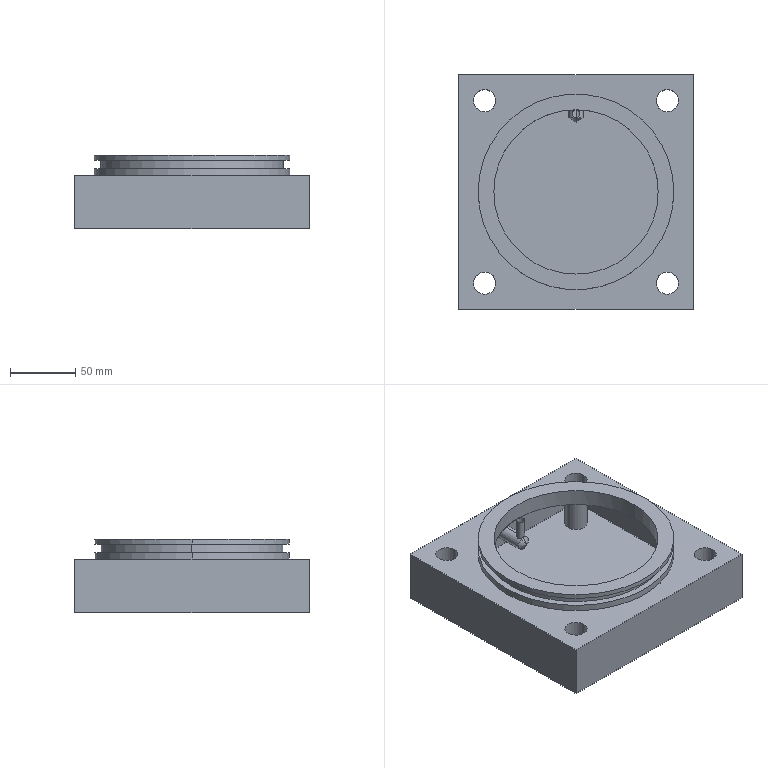Part | SolidWorks | features ICE 4, Extrusion 1, HoleWzd 1, RevCut 1 | 1 solid | 35 faces | box 180 x 180 x 56 mm | volume 1375420 mm3 | cylinder 20 | plane 11 | cone 4 | commonest cylinder face diameters 17 x8 150 x4 6 x2 11.125 x2 126 x2 140 x2
STEP:
#1=CARTESIAN_POINT('',(61.5,-70.,41.));
#2=VERTEX_POINT('',#1);
#3=CARTESIAN_POINT('',(78.5,-70.,41.));
#4=VERTEX_POINT('',#3);
#5=CARTESIAN_POINT('',(70.,-70.,41.));
#6=DIRECTION('',(0.,0.,1.));
#7=DIRECTION('',(-1.,0.,0.));
#8=AXIS2_PLACEMENT_3D('',#5,#6,#7);
#9=CIRCLE('',#8,8.5);
#10=EDGE_CURVE('',#2,#4,#9,.T.);
#11=ORIENTED_EDGE('',*,*,#10,.T.);
#12=CARTESIAN_POINT('',(78.5,-70.,0.));
#13=VERTEX_POINT('',#12);
#14=CARTESIAN_POINT('',(78.5,-70.,56.001));
#15=DIRECTION('',(0.,0.,-1.));
#16=VECTOR('',#15,1000.);
#17=LINE('',#14,#16);
#18=EDGE_CURVE('',#4,#13,#17,.T.);
#19=ORIENTED_EDGE('',*,*,#18,.T.);
#20=CARTESIAN_POINT('',(61.5,-70.,0.));
#21=VERTEX_POINT('',#20);
#22=CARTESIAN_POINT('',(70.,-70.,0.));
#23=DIRECTION('',(0.,0.,-1.));
#24=DIRECTION('',(-1.,0.,0.));
#25=AXIS2_PLACEMENT_3D('',#22,#23,#24);
#26=CIRCLE('',#25,8.5);
#27=EDGE_CURVE('',#13,#21,#26,.T.);
#28=ORIENTED_EDGE('',*,*,#27,.T.);
#29=CARTESIAN_POINT('',(61.5,-70.,56.001));
#30=DIRECTION('',(0.,0.,-1.));
#31=VECTOR('',#30,1000.);
#32=LINE('',#29,#31);
#33=EDGE_CURVE('',#2,#21,#32,.T.);
#34=ORIENTED_EDGE('',*,*,#33,.F.);
#35=EDGE_LOOP('',(#11,#19,#28,#34));
#36=FACE_OUTER_BOUND('',#35,.T.);
#37=CARTESIAN_POINT('',(70.,-70.,56.001));
#38=DIRECTION('',(0.,0.,-1.));
#39=DIRECTION('',(-1.,0.,0.));
#40=AXIS2_PLACEMENT_3D('',#37,#38,#39);
#41=CYLINDRICAL_SURFACE('',#40,8.5);
#42=ADVANCED_FACE('',(#36),#41,.F.);
#43=CARTESIAN_POINT('',(-78.5,-70.,41.));
#44=VERTEX_POINT('',#43);
#45=CARTESIAN_POINT('',(-61.5,-70.,41.));
#46=VERTEX_POINT('',#45);
#47=CARTESIAN_POINT('',(-70.,-70.,41.));
#48=DIRECTION('',(0.,0.,1.));
#49=DIRECTION('',(-1.,0.,0.));
#50=AXIS2_PLACEMENT_3D('',#47,#48,#49);
#51=CIRCLE('',#50,8.5);
#52=EDGE_CURVE('',#44,#46,#51,.T.);
#53=ORIENTED_EDGE('',*,*,#52,.T.);
#54=CARTESIAN_POINT('',(-61.5,-70.,0.));
#55=VERTEX_POINT('',#54);
#56=CARTESIAN_POINT('',(-61.5,-70.,56.001));
#57=DIRECTION('',(0.,0.,-1.));
#58=VECTOR('',#57,1000.);
#59=LINE('',#56,#58);
#60=EDGE_CURVE('',#46,#55,#59,.T.);
#61=ORIENTED_EDGE('',*,*,#60,.T.);
#62=CARTESIAN_POINT('',(-78.5,-70.,0.));
#63=VERTEX_POINT('',#62);
#64=CARTESIAN_POINT('',(-70.,-70.,0.));
#65=DIRECTION('',(0.,0.,-1.));
#66=DIRECTION('',(-1.,0.,0.));
#67=AXIS2_PLACEMENT_3D('',#64,#65,#66);
#68=CIRCLE('',#67,8.5);
#69=EDGE_CURVE('',#55,#63,#68,.T.);
#70=ORIENTED_EDGE('',*,*,#69,.T.);
#71=CARTESIAN_POINT('',(-78.5,-70.,56.001));
#72=DIRECTION('',(0.,0.,-1.));
#73=VECTOR('',#72,1000.);
#74=LINE('',#71,#73);
#75=EDGE_CURVE('',#44,#63,#74,.T.);
#76=ORIENTED_EDGE('',*,*,#75,.F.);
#77=EDGE_LOOP('',(#53,#61,#70,#76));
#78=FACE_OUTER_BOUND('',#77,.T.);
#79=CARTESIAN_POINT('',(-70.,-70.,56.001));
#80=DIRECTION('',(0.,0.,-1.));
#81=DIRECTION('',(-1.,0.,0.));
#82=AXIS2_PLACEMENT_3D('',#79,#80,#81);
#83=CYLINDRICAL_SURFACE('',#82,8.5);
#84=ADVANCED_FACE('',(#78),#83,.F.);
#85=CARTESIAN_POINT('',(-78.5,70.,41.));
#86=VERTEX_POINT('',#85);
#87=CARTESIAN_POINT('',(-61.5,70.,41.));
#88=VERTEX_POINT('',#87);
#89=CARTESIAN_POINT('',(-70.,70.,41.));
#90=DIRECTION('',(0.,0.,1.));
#91=DIRECTION('',(-1.,0.,0.));
#92=AXIS2_PLACEMENT_3D('',#89,#90,#91);
#93=CIRCLE('',#92,8.5);
#94=EDGE_CURVE('',#86,#88,#93,.T.);
#95=ORIENTED_EDGE('',*,*,#94,.T.);
#96=CARTESIAN_POINT('',(-61.5,70.,0.));
#97=VERTEX_POINT('',#96);
#98=CARTESIAN_POINT('',(-61.5,70.,56.001));
#99=DIRECTION('',(0.,0.,-1.));
#100=VECTOR('',#99,1000.);
#101=LINE('',#98,#100);
#102=EDGE_CURVE('',#88,#97,#101,.T.);
#103=ORIENTED_EDGE('',*,*,#102,.T.);
#104=CARTESIAN_POINT('',(-78.5,70.,0.));
#105=VERTEX_POINT('',#104);
#106=CARTESIAN_POINT('',(-70.,70.,0.));
#107=DIRECTION('',(0.,0.,-1.));
#108=DIRECTION('',(-1.,0.,0.));
#109=AXIS2_PLACEMENT_3D('',#106,#107,#108);
#110=CIRCLE('',#109,8.5);
#111=EDGE_CURVE('',#97,#105,#110,.T.);
#112=ORIENTED_EDGE('',*,*,#111,.T.);
#113=CARTESIAN_POINT('',(-78.5,70.,56.001));
#114=DIRECTION('',(0.,0.,-1.));
#115=VECTOR('',#114,1000.);
#116=LINE('',#113,#115);
#117=EDGE_CURVE('',#86,#105,#116,.T.);
#118=ORIENTED_EDGE('',*,*,#117,.F.);
#119=EDGE_LOOP('',(#95,#103,#112,#118));
#120=FACE_OUTER_BOUND('',#119,.T.);
#121=CARTESIAN_POINT('',(-70.,70.,56.001));
#122=DIRECTION('',(0.,0.,-1.));
#123=DIRECTION('',(-1.,0.,0.));
#124=AXIS2_PLACEMENT_3D('',#121,#122,#123);
#125=CYLINDRICAL_SURFACE('',#124,8.5);
#126=ADVANCED_FACE('',(#120),#125,.F.);
#127=CARTESIAN_POINT('',(61.5,70.,41.));
#128=VERTEX_POINT('',#127);
#129=CARTESIAN_POINT('',(78.5,70.,41.));
#130=VERTEX_POINT('',#129);
#131=CARTESIAN_POINT('',(70.,70.,41.));
#132=DIRECTION('',(0.,0.,1.));
#133=DIRECTION('',(-1.,0.,0.));
#134=AXIS2_PLACEMENT_3D('',#131,#132,#133);
#135=CIRCLE('',#134,8.5);
#136=EDGE_CURVE('',#128,#130,#135,.T.);
#137=ORIENTED_EDGE('',*,*,#136,.T.);
#138=CARTESIAN_POINT('',(78.5,70.,0.));
#139=VERTEX_POINT('',#138);
#140=CARTESIAN_POINT('',(78.5,70.,56.001));
#141=DIRECTION('',(0.,0.,-1.));
#142=VECTOR('',#141,1000.);
#143=LINE('',#140,#142);
#144=EDGE_CURVE('',#130,#139,#143,.T.);
#145=ORIENTED_EDGE('',*,*,#144,.T.);
#146=CARTESIAN_POINT('',(61.5,70.,0.));
#147=VERTEX_POINT('',#146);
#148=CARTESIAN_POINT('',(70.,70.,0.));
#149=DIRECTION('',(0.,0.,-1.));
#150=DIRECTION('',(-1.,0.,0.));
#151=AXIS2_PLACEMENT_3D('',#148,#149,#150);
#152=CIRCLE('',#151,8.5);
#153=EDGE_CURVE('',#139,#147,#152,.T.);
#154=ORIENTED_EDGE('',*,*,#153,.T.);
#155=CARTESIAN_POINT('',(61.5,70.,56.001));
#156=DIRECTION('',(0.,0.,-1.));
#157=VECTOR('',#156,1000.);
#158=LINE('',#155,#157);
#159=EDGE_CURVE('',#128,#147,#158,.T.);
#160=ORIENTED_EDGE('',*,*,#159,.F.);
#161=EDGE_LOOP('',(#137,#145,#154,#160));
#162=FACE_OUTER_BOUND('',#161,.T.);
#163=CARTESIAN_POINT('',(70.,70.,56.001));
#164=DIRECTION('',(0.,0.,-1.));
#165=DIRECTION('',(-1.,0.,0.));
#166=AXIS2_PLACEMENT_3D('',#163,#164,#165);
#167=CYLINDRICAL_SURFACE('',#166,8.5);
#168=ADVANCED_FACE('',(#162),#167,.F.);
#169=CARTESIAN_POINT('',(0.,57.,28.563));
#170=VERTEX_POINT('',#169);
#171=CARTESIAN_POINT('',(-3.,60.,27.684));
#172=VERTEX_POINT('',#171);
#173=CARTESIAN_POINT('',(0.,57.,28.563));
#174=CARTESIAN_POINT('',(-0.2027,57.,28.563));
#175=CARTESIAN_POINT('',(-0.4013,57.02,28.552));
#176=CARTESIAN_POINT('',(-0.7909,57.099,28.51));
#177=CARTESIAN_POINT('',(-0.9837,57.159,28.478));
#178=CARTESIAN_POINT('',(-1.527,57.388,28.362));
#179=CARTESIAN_POINT('',(-1.855,57.611,28.253));
#180=CARTESIAN_POINT('',(-2.261,58.019,28.084));
#181=CARTESIAN_POINT('',(-2.385,58.169,28.027));
#182=CARTESIAN_POINT('',(-2.6,58.491,27.919));
#183=CARTESIAN_POINT('',(-2.692,58.661,27.869));
#184=CARTESIAN_POINT('',(-2.842,59.02,27.782));
#185=CARTESIAN_POINT('',(-2.902,59.213,27.746));
#186=CARTESIAN_POINT('',(-2.98,59.602,27.697));
#187=CARTESIAN_POINT('',(-3.,59.799,27.684));
#188=CARTESIAN_POINT('',(-3.,60.,27.684));
#189=B_SPLINE_CURVE_WITH_KNOTS('',3,(#173,#174,#175,#176,#177,#178,#179,#180,#181,#182,#183,#184,#185,#186,#187,#188),.UNSPECIFIED.,.F.,.F.,(4,2,2,2,2,2,2,4),(0.,0.0005988,0.001198,0.002395,0.002994,0.003593,0.004192,0.00479),.UNSPECIFIED.);
#190=EDGE_CURVE('',#170,#172,#189,.T.);
#191=ORIENTED_EDGE('',*,*,#190,.T.);
#192=CARTESIAN_POINT('',(-3.,60.,43.));
#193=VERTEX_POINT('',#192);
#194=CARTESIAN_POINT('',(-3.,60.,-0.001));
#195=DIRECTION('',(0.,0.,1.));
#196=VECTOR('',#195,1000.);
#197=LINE('',#194,#196);
#198=EDGE_CURVE('',#172,#193,#197,.T.);
#199=ORIENTED_EDGE('',*,*,#198,.T.);
#200=CARTESIAN_POINT('',(3.,60.,43.));
#201=VERTEX_POINT('',#200);
#202=CARTESIAN_POINT('',(0.,60.,43.));
#203=DIRECTION('',(0.,0.,1.));
#204=DIRECTION('',(1.,0.,0.));
#205=AXIS2_PLACEMENT_3D('',#202,#203,#204);
#206=CIRCLE('',#205,3.);
#207=EDGE_CURVE('',#193,#201,#206,.T.);
#208=ORIENTED_EDGE('',*,*,#207,.T.);
#209=CARTESIAN_POINT('',(3.,60.,27.684));
#210=VERTEX_POINT('',#209);
#211=CARTESIAN_POINT('',(3.,60.,-0.001));
#212=DIRECTION('',(0.,0.,1.));
#213=VECTOR('',#212,1000.);
#214=LINE('',#211,#213);
#215=EDGE_CURVE('',#210,#201,#214,.T.);
#216=ORIENTED_EDGE('',*,*,#215,.F.);
#217=CARTESIAN_POINT('',(3.,60.,27.684));
#218=CARTESIAN_POINT('',(3.,59.801,27.684));
#219=CARTESIAN_POINT('',(2.98,59.598,27.697));
#220=CARTESIAN_POINT('',(2.901,59.209,27.747));
#221=CARTESIAN_POINT('',(2.843,59.021,27.782));
#222=CARTESIAN_POINT('',(2.69,58.657,27.87));
#223=CARTESIAN_POINT('',(2.597,58.486,27.92));
#224=CARTESIAN_POINT('',(2.382,58.167,28.028));
#225=CARTESIAN_POINT('',(2.258,58.016,28.086));
#226=CARTESIAN_POINT('',(1.987,57.744,28.198));
#227=CARTESIAN_POINT('',(1.839,57.622,28.252));
#228=CARTESIAN_POINT('',(1.518,57.405,28.354));
#229=CARTESIAN_POINT('',(1.344,57.311,28.401));
#230=CARTESIAN_POINT('',(0.9842,57.159,28.478));
#231=CARTESIAN_POINT('',(0.7966,57.101,28.509));
#232=CARTESIAN_POINT('',(0.4039,57.021,28.551));
#233=CARTESIAN_POINT('',(0.2019,57.,28.563));
#234=CARTESIAN_POINT('',(0.,57.,28.563));
#235=B_SPLINE_CURVE_WITH_KNOTS('',3,(#217,#218,#219,#220,#221,#222,#223,#224,#225,#226,#227,#228,#229,#230,#231,#232,#233,#234),.UNSPECIFIED.,.F.,.F.,(4,2,2,2,2,2,2,2,4),(0.01435,0.01495,0.01555,0.01614,0.01674,0.01734,0.01793,0.01853,0.01913),.UNSPECIFIED.);
#236=EDGE_CURVE('',#210,#170,#235,.T.);
#237=ORIENTED_EDGE('',*,*,#236,.T.);
#238=EDGE_LOOP('',(#191,#199,#208,#216,#237));
#239=FACE_OUTER_BOUND('',#238,.T.);
#240=CARTESIAN_POINT('',(0.,60.,-0.001));
#241=DIRECTION('',(0.,0.,1.));
#242=DIRECTION('',(1.,0.,0.));
#243=AXIS2_PLACEMENT_3D('',#240,#241,#242);
#244=CYLINDRICAL_SURFACE('',#243,3.);
#245=ADVANCED_FACE('',(#239),#244,.F.);
#246=CARTESIAN_POINT('',(0.,79.98,17.056));
#247=VERTEX_POINT('',#246);
#248=CARTESIAN_POINT('',(0.,79.98,28.944));
#249=VERTEX_POINT('',#248);
#250=CARTESIAN_POINT('',(0.,79.98,23.));
#251=DIRECTION('',(0.,1.,0.));
#252=DIRECTION('',(0.,0.,1.));
#253=AXIS2_PLACEMENT_3D('',#250,#251,#252);
#254=CIRCLE('',#253,5.944);
#255=EDGE_CURVE('',#247,#249,#254,.T.);
#256=ORIENTED_EDGE('',*,*,#255,.F.);
#257=CARTESIAN_POINT('',(0.,90.,16.756));
#258=VERTEX_POINT('',#257);
#259=CARTESIAN_POINT('',(0.,90.,16.756));
#260=DIRECTION('',(0.,0.9996,-0.02993));
#261=VECTOR('',#260,1000.);
#262=LINE('',#259,#261);
#263=EDGE_CURVE('',#247,#258,#262,.T.);
#264=ORIENTED_EDGE('',*,*,#263,.T.);
#265=CARTESIAN_POINT('',(0.,90.,29.244));
#266=VERTEX_POINT('',#265);
#267=CARTESIAN_POINT('',(0.,90.,23.));
#268=DIRECTION('',(0.,1.,0.));
#269=DIRECTION('',(0.,0.,1.));
#270=AXIS2_PLACEMENT_3D('',#267,#268,#269);
#271=CIRCLE('',#270,6.244);
#272=EDGE_CURVE('',#258,#266,#271,.T.);
#273=ORIENTED_EDGE('',*,*,#272,.T.);
#274=CARTESIAN_POINT('',(0.,90.,29.244));
#275=DIRECTION('',(0.,0.9996,0.02993));
#276=VECTOR('',#275,1000.);
#277=LINE('',#274,#276);
#278=EDGE_CURVE('',#249,#266,#277,.T.);
#279=ORIENTED_EDGE('',*,*,#278,.F.);
#280=EDGE_LOOP('',(#256,#264,#273,#279));
#281=FACE_OUTER_BOUND('',#280,.T.);
#282=CARTESIAN_POINT('',(0.,90.,23.));
#283=DIRECTION('',(0.,1.,0.));
#284=DIRECTION('',(0.,0.,1.));
#285=AXIS2_PLACEMENT_3D('',#282,#283,#284);
#286=CONICAL_SURFACE('',#285,6.244,0.02993);
#287=ADVANCED_FACE('',(#281),#286,.F.);
#288=CARTESIAN_POINT('',(0.,57.,17.437));
#289=VERTEX_POINT('',#288);
#290=CARTESIAN_POINT('',(0.,57.,23.));
#291=DIRECTION('',(0.,1.,0.));
#292=DIRECTION('',(0.,0.,1.));
#293=AXIS2_PLACEMENT_3D('',#290,#291,#292);
#294=CIRCLE('',#293,5.563);
#295=EDGE_CURVE('',#289,#170,#294,.T.);
#296=ORIENTED_EDGE('',*,*,#295,.F.);
#297=CARTESIAN_POINT('',(0.,79.98,17.437));
#298=VERTEX_POINT('',#297);
#299=CARTESIAN_POINT('',(0.,90.,17.437));
#300=DIRECTION('',(0.,1.,0.));
#301=VECTOR('',#300,1000.);
#302=LINE('',#299,#301);
#303=EDGE_CURVE('',#289,#298,#302,.T.);
#304=ORIENTED_EDGE('',*,*,#303,.T.);
#305=CARTESIAN_POINT('',(0.,79.98,28.563));
#306=VERTEX_POINT('',#305);
#307=CARTESIAN_POINT('',(0.,79.98,23.));
#308=DIRECTION('',(0.,1.,0.));
#309=DIRECTION('',(0.,0.,1.));
#310=AXIS2_PLACEMENT_3D('',#307,#308,#309);
#311=CIRCLE('',#310,5.563);
#312=EDGE_CURVE('',#298,#306,#311,.T.);
#313=ORIENTED_EDGE('',*,*,#312,.T.);
#314=CARTESIAN_POINT('',(0.,63.,28.563));
#315=VERTEX_POINT('',#314);
#316=CARTESIAN_POINT('',(0.,90.,28.563));
#317=DIRECTION('',(0.,1.,0.));
#318=VECTOR('',#317,1000.);
#319=LINE('',#316,#318);
#320=EDGE_CURVE('',#315,#306,#319,.T.);
#321=ORIENTED_EDGE('',*,*,#320,.F.);
#322=CARTESIAN_POINT('',(-3.,60.,27.684));
#323=CARTESIAN_POINT('',(-3.,60.2,27.684));
#324=CARTESIAN_POINT('',(-2.979,60.403,27.698));
#325=CARTESIAN_POINT('',(-2.9,60.792,27.747));
#326=CARTESIAN_POINT('',(-2.841,60.982,27.783));
#327=CARTESIAN_POINT('',(-2.689,61.344,27.87));
#328=CARTESIAN_POINT('',(-2.597,61.515,27.921));
#329=CARTESIAN_POINT('',(-2.38,61.836,28.029));
#330=CARTESIAN_POINT('',(-2.257,61.986,28.086));
#331=CARTESIAN_POINT('',(-1.85,62.393,28.254));
#332=CARTESIAN_POINT('',(-1.522,62.615,28.363));
#333=CARTESIAN_POINT('',(-0.9815,62.842,28.478));
#334=CARTESIAN_POINT('',(-0.7896,62.901,28.51));
#335=CARTESIAN_POINT('',(-0.398,62.98,28.552));
#336=CARTESIAN_POINT('',(-0.2001,63.,28.563));
#337=CARTESIAN_POINT('',(0.,63.,28.563));
#338=B_SPLINE_CURVE_WITH_KNOTS('',3,(#322,#323,#324,#325,#326,#327,#328,#329,#330,#331,#332,#333,#334,#335,#336,#337),.UNSPECIFIED.,.F.,.F.,(4,2,2,2,2,2,2,4),(0.00479,0.005388,0.005986,0.006584,0.007182,0.008378,0.008976,0.009574),.UNSPECIFIED.);
#339=EDGE_CURVE('',#172,#315,#338,.T.);
#340=ORIENTED_EDGE('',*,*,#339,.F.);
#341=ORIENTED_EDGE('',*,*,#190,.F.);
#342=EDGE_LOOP('',(#296,#304,#313,#321,#340,#341));
#343=FACE_OUTER_BOUND('',#342,.T.);
#344=CARTESIAN_POINT('',(0.,90.,23.));
#345=DIRECTION('',(0.,1.,0.));
#346=DIRECTION('',(0.,0.,1.));
#347=AXIS2_PLACEMENT_3D('',#344,#345,#346);
#348=CYLINDRICAL_SURFACE('',#347,5.563);
#349=ADVANCED_FACE('',(#343),#348,.F.);
#350=CARTESIAN_POINT('',(0.,53.658,23.));
#351=VERTEX_POINT('',#350);
#352=CARTESIAN_POINT('',(0.,57.,28.563));
#353=DIRECTION('',(0.,0.515,0.8572));
#354=VECTOR('',#353,1000.);
#355=LINE('',#352,#354);
#356=EDGE_CURVE('',#351,#170,#355,.T.);
#357=ORIENTED_EDGE('',*,*,#356,.F.);
#358=CARTESIAN_POINT('',(0.,57.,17.437));
#359=DIRECTION('',(0.,0.515,-0.8572));
#360=VECTOR('',#359,1000.);
#361=LINE('',#358,#360);
#362=EDGE_CURVE('',#351,#289,#361,.T.);
#363=ORIENTED_EDGE('',*,*,#362,.T.);
#364=ORIENTED_EDGE('',*,*,#295,.T.);
#365=EDGE_LOOP('',(#357,#363,#364));
#366=FACE_OUTER_BOUND('',#365,.T.);
#367=CARTESIAN_POINT('',(0.,57.,23.));
#368=DIRECTION('',(0.,1.,0.));
#369=DIRECTION('',(0.,0.,1.));
#370=AXIS2_PLACEMENT_3D('',#367,#368,#369);
#371=CONICAL_SURFACE('',#370,5.563,1.03);
#372=ADVANCED_FACE('',(#366),#371,.F.);
#373=CARTESIAN_POINT('',(75.,0.,46.));
#374=VERTEX_POINT('',#373);
#375=CARTESIAN_POINT('',(-75.,0.,46.));
#376=VERTEX_POINT('',#375);
#377=CARTESIAN_POINT('',(0.,0.,46.));
#378=DIRECTION('',(0.,0.,1.));
#379=DIRECTION('',(1.,0.,0.));
#380=AXIS2_PLACEMENT_3D('',#377,#378,#379);
#381=CIRCLE('',#380,75.);
#382=EDGE_CURVE('',#374,#376,#381,.T.);
#383=ORIENTED_EDGE('',*,*,#382,.F.);
#384=CARTESIAN_POINT('',(75.,0.,41.));
#385=VERTEX_POINT('',#384);
#386=CARTESIAN_POINT('',(75.,0.,56.));
#387=DIRECTION('',(0.,0.,-1.));
#388=VECTOR('',#387,1000.);
#389=LINE('',#386,#388);
#390=EDGE_CURVE('',#374,#385,#389,.T.);
#391=ORIENTED_EDGE('',*,*,#390,.T.);
#392=CARTESIAN_POINT('',(-75.,0.,41.));
#393=VERTEX_POINT('',#392);
#394=CARTESIAN_POINT('',(0.,0.,41.));
#395=DIRECTION('',(0.,0.,1.));
#396=DIRECTION('',(1.,0.,0.));
#397=AXIS2_PLACEMENT_3D('',#394,#395,#396);
#398=CIRCLE('',#397,75.);
#399=EDGE_CURVE('',#385,#393,#398,.T.);
#400=ORIENTED_EDGE('',*,*,#399,.T.);
#401=CARTESIAN_POINT('',(-75.,0.,56.));
#402=DIRECTION('',(0.,0.,-1.));
#403=VECTOR('',#402,1000.);
#404=LINE('',#401,#403);
#405=EDGE_CURVE('',#376,#393,#404,.T.);
#406=ORIENTED_EDGE('',*,*,#405,.F.);
#407=EDGE_LOOP('',(#383,#391,#400,#406));
#408=FACE_OUTER_BOUND('',#407,.T.);
#409=CARTESIAN_POINT('',(0.,0.,56.));
#410=DIRECTION('',(0.,0.,-1.));
#411=DIRECTION('',(-1.,0.,0.));
#412=AXIS2_PLACEMENT_3D('',#409,#410,#411);
#413=CYLINDRICAL_SURFACE('',#412,75.);
#414=ADVANCED_FACE('',(#408),#413,.T.);
#415=CARTESIAN_POINT('',(70.,0.,46.));
#416=VERTEX_POINT('',#415);
#417=CARTESIAN_POINT('',(-70.,0.,46.));
#418=VERTEX_POINT('',#417);
#419=CARTESIAN_POINT('',(0.,0.,46.));
#420=DIRECTION('',(0.,0.,1.));
#421=DIRECTION('',(1.,0.,0.));
#422=AXIS2_PLACEMENT_3D('',#419,#420,#421);
#423=CIRCLE('',#422,70.);
#424=EDGE_CURVE('',#416,#418,#423,.T.);
#425=ORIENTED_EDGE('',*,*,#424,.T.);
#426=CARTESIAN_POINT('',(-70.,0.,52.5));
#427=VERTEX_POINT('',#426);
#428=CARTESIAN_POINT('',(-70.,0.,56.));
#429=DIRECTION('',(0.,0.,1.));
#430=VECTOR('',#429,1000.);
#431=LINE('',#428,#430);
#432=EDGE_CURVE('',#418,#427,#431,.T.);
#433=ORIENTED_EDGE('',*,*,#432,.T.);
#434=CARTESIAN_POINT('',(70.,0.,52.5));
#435=VERTEX_POINT('',#434);
#436=CARTESIAN_POINT('',(0.,0.,52.5));
#437=DIRECTION('',(0.,0.,1.));
#438=DIRECTION('',(1.,0.,0.));
#439=AXIS2_PLACEMENT_3D('',#436,#437,#438);
#440=CIRCLE('',#439,70.);
#441=EDGE_CURVE('',#435,#427,#440,.T.);
#442=ORIENTED_EDGE('',*,*,#441,.F.);
#443=CARTESIAN_POINT('',(70.,0.,56.));
#444=DIRECTION('',(0.,0.,1.));
#445=VECTOR('',#444,1000.);
#446=LINE('',#443,#445);
#447=EDGE_CURVE('',#416,#435,#446,.T.);
#448=ORIENTED_EDGE('',*,*,#447,.F.);
#449=EDGE_LOOP('',(#425,#433,#442,#448));
#450=FACE_OUTER_BOUND('',#449,.T.);
#451=CARTESIAN_POINT('',(0.,0.,56.));
#452=DIRECTION('',(0.,0.,1.));
#453=DIRECTION('',(1.,0.,0.));
#454=AXIS2_PLACEMENT_3D('',#451,#452,#453);
#455=CYLINDRICAL_SURFACE('',#454,70.);
#456=ADVANCED_FACE('',(#450),#455,.T.);
#457=CARTESIAN_POINT('',(-63.,0.,43.));
#458=VERTEX_POINT('',#457);
#459=CARTESIAN_POINT('',(63.,0.,43.));
#460=VERTEX_POINT('',#459);
#461=CARTESIAN_POINT('',(0.,0.,43.));
#462=DIRECTION('',(0.,0.,1.));
#463=DIRECTION('',(1.,0.,0.));
#464=AXIS2_PLACEMENT_3D('',#461,#462,#463);
#465=CIRCLE('',#464,63.);
#466=EDGE_CURVE('',#458,#460,#465,.T.);
#467=ORIENTED_EDGE('',*,*,#466,.F.);
#468=CARTESIAN_POINT('',(-63.,0.,56.));
#469=VERTEX_POINT('',#468);
#470=CARTESIAN_POINT('',(-63.,0.,43.));
#471=DIRECTION('',(0.,0.,1.));
#472=VECTOR('',#471,1000.);
#473=LINE('',#470,#472);
#474=EDGE_CURVE('',#458,#469,#473,.T.);
#475=ORIENTED_EDGE('',*,*,#474,.T.);
#476=CARTESIAN_POINT('',(63.,0.,56.));
#477=VERTEX_POINT('',#476);
#478=CARTESIAN_POINT('',(0.,0.,56.));
#479=DIRECTION('',(0.,0.,1.));
#480=DIRECTION('',(1.,0.,0.));
#481=AXIS2_PLACEMENT_3D('',#478,#479,#480);
#482=CIRCLE('',#481,63.);
#483=EDGE_CURVE('',#469,#477,#482,.T.);
#484=ORIENTED_EDGE('',*,*,#483,.T.);
#485=CARTESIAN_POINT('',(63.,0.,43.));
#486=DIRECTION('',(0.,0.,1.));
#487=VECTOR('',#486,1000.);
#488=LINE('',#485,#487);
#489=EDGE_CURVE('',#460,#477,#488,.T.);
#490=ORIENTED_EDGE('',*,*,#489,.F.);
#491=EDGE_LOOP('',(#467,#475,#484,#490));
#492=FACE_OUTER_BOUND('',#491,.T.);
#493=CARTESIAN_POINT('',(0.,0.,43.));
#494=DIRECTION('',(0.,0.,1.));
#495=DIRECTION('',(1.,0.,0.));
#496=AXIS2_PLACEMENT_3D('',#493,#494,#495);
#497=CYLINDRICAL_SURFACE('',#496,63.);
#498=ADVANCED_FACE('',(#492),#497,.F.);
#499=CARTESIAN_POINT('',(75.,0.,56.));
#500=VERTEX_POINT('',#499);
#501=CARTESIAN_POINT('',(-75.,0.,56.));
#502=VERTEX_POINT('',#501);
#503=CARTESIAN_POINT('',(0.,0.,56.));
#504=DIRECTION('',(0.,0.,1.));
#505=DIRECTION('',(1.,0.,0.));
#506=AXIS2_PLACEMENT_3D('',#503,#504,#505);
#507=CIRCLE('',#506,75.);
#508=EDGE_CURVE('',#500,#502,#507,.T.);
#509=ORIENTED_EDGE('',*,*,#508,.F.);
#510=CARTESIAN_POINT('',(75.,0.,52.5));
#511=VERTEX_POINT('',#510);
#512=CARTESIAN_POINT('',(75.,0.,56.));
#513=DIRECTION('',(0.,0.,-1.));
#514=VECTOR('',#513,1000.);
#515=LINE('',#512,#514);
#516=EDGE_CURVE('',#500,#511,#515,.T.);
#517=ORIENTED_EDGE('',*,*,#516,.T.);
#518=CARTESIAN_POINT('',(-75.,0.,52.5));
#519=VERTEX_POINT('',#518);
#520=CARTESIAN_POINT('',(0.,0.,52.5));
#521=DIRECTION('',(0.,0.,1.));
#522=DIRECTION('',(1.,0.,0.));
#523=AXIS2_PLACEMENT_3D('',#520,#521,#522);
#524=CIRCLE('',#523,75.);
#525=EDGE_CURVE('',#511,#519,#524,.T.);
#526=ORIENTED_EDGE('',*,*,#525,.T.);
#527=CARTESIAN_POINT('',(-75.,0.,56.));
#528=DIRECTION('',(0.,0.,-1.));
#529=VECTOR('',#528,1000.);
#530=LINE('',#527,#529);
#531=EDGE_CURVE('',#502,#519,#530,.T.);
#532=ORIENTED_EDGE('',*,*,#531,.F.);
#533=EDGE_LOOP('',(#509,#517,#526,#532));
#534=FACE_OUTER_BOUND('',#533,.T.);
#535=CARTESIAN_POINT('',(0.,0.,56.));
#536=DIRECTION('',(0.,0.,-1.));
#537=DIRECTION('',(-1.,0.,0.));
#538=AXIS2_PLACEMENT_3D('',#535,#536,#537);
#539=CYLINDRICAL_SURFACE('',#538,75.);
#540=ADVANCED_FACE('',(#534),#539,.T.);
#541=ORIENTED_EDGE('',*,*,#516,.F.);
#542=CARTESIAN_POINT('',(0.,0.,56.));
#543=DIRECTION('',(0.,0.,1.));
#544=DIRECTION('',(1.,0.,0.));
#545=AXIS2_PLACEMENT_3D('',#542,#543,#544);
#546=CIRCLE('',#545,75.);
#547=EDGE_CURVE('',#502,#500,#546,.T.);
#548=ORIENTED_EDGE('',*,*,#547,.F.);
#549=ORIENTED_EDGE('',*,*,#531,.T.);
#550=CARTESIAN_POINT('',(0.,0.,52.5));
#551=DIRECTION('',(0.,0.,1.));
#552=DIRECTION('',(1.,0.,0.));
#553=AXIS2_PLACEMENT_3D('',#550,#551,#552);
#554=CIRCLE('',#553,75.);
#555=EDGE_CURVE('',#519,#511,#554,.T.);
#556=ORIENTED_EDGE('',*,*,#555,.T.);
#557=EDGE_LOOP('',(#541,#548,#549,#556));
#558=FACE_OUTER_BOUND('',#557,.T.);
#559=CARTESIAN_POINT('',(0.,0.,56.));
#560=DIRECTION('',(0.,0.,-1.));
#561=DIRECTION('',(-1.,0.,0.));
#562=AXIS2_PLACEMENT_3D('',#559,#560,#561);
#563=CYLINDRICAL_SURFACE('',#562,75.);
#564=ADVANCED_FACE('',(#558),#563,.T.);
#565=CARTESIAN_POINT('',(0.,0.,56.));
#566=DIRECTION('',(0.,0.,1.));
#567=DIRECTION('',(1.,0.,0.));
#568=AXIS2_PLACEMENT_3D('',#565,#566,#567);
#569=CIRCLE('',#568,63.);
#570=EDGE_CURVE('',#477,#469,#569,.T.);
#571=ORIENTED_EDGE('',*,*,#570,.F.);
#572=ORIENTED_EDGE('',*,*,#483,.F.);
#573=EDGE_LOOP('',(#571,#572));
#574=FACE_BOUND('',#573,.T.);
#575=ORIENTED_EDGE('',*,*,#547,.T.);
#576=ORIENTED_EDGE('',*,*,#508,.T.);
#577=EDGE_LOOP('',(#575,#576));
#578=FACE_OUTER_BOUND('',#577,.T.);
#579=CARTESIAN_POINT('',(0.,0.,56.));
#580=DIRECTION('',(0.,0.,1.));
#581=DIRECTION('',(1.,0.,0.));
#582=AXIS2_PLACEMENT_3D('',#579,#580,#581);
#583=PLANE('',#582);
#584=ADVANCED_FACE('',(#574,#578),#583,.T.);
#585=ORIENTED_EDGE('',*,*,#474,.F.);
#586=CARTESIAN_POINT('',(0.,63.,43.));
#587=VERTEX_POINT('',#586);
#588=CARTESIAN_POINT('',(0.,0.,43.));
#589=DIRECTION('',(0.,0.,1.));
#590=DIRECTION('',(1.,0.,0.));
#591=AXIS2_PLACEMENT_3D('',#588,#589,#590);
#592=CIRCLE('',#591,63.);
#593=EDGE_CURVE('',#587,#458,#592,.T.);
#594=ORIENTED_EDGE('',*,*,#593,.F.);
#595=CARTESIAN_POINT('',(0.,0.,43.));
#596=DIRECTION('',(0.,0.,1.));
#597=DIRECTION('',(1.,0.,0.));
#598=AXIS2_PLACEMENT_3D('',#595,#596,#597);
#599=CIRCLE('',#598,63.);
#600=EDGE_CURVE('',#460,#587,#599,.T.);
#601=ORIENTED_EDGE('',*,*,#600,.F.);
#602=ORIENTED_EDGE('',*,*,#489,.T.);
#603=ORIENTED_EDGE('',*,*,#570,.T.);
#604=EDGE_LOOP('',(#585,#594,#601,#602,#603));
#605=FACE_OUTER_BOUND('',#604,.T.);
#606=CARTESIAN_POINT('',(0.,0.,43.));
#607=DIRECTION('',(0.,0.,1.));
#608=DIRECTION('',(1.,0.,0.));
#609=AXIS2_PLACEMENT_3D('',#606,#607,#608);
#610=CYLINDRICAL_SURFACE('',#609,63.);
#611=ADVANCED_FACE('',(#605),#610,.F.);
#612=ORIENTED_EDGE('',*,*,#593,.T.);
#613=ORIENTED_EDGE('',*,*,#466,.T.);
#614=ORIENTED_EDGE('',*,*,#600,.T.);
#615=CARTESIAN_POINT('',(0.,60.,43.));
#616=DIRECTION('',(0.,0.,1.));
#617=DIRECTION('',(1.,0.,0.));
#618=AXIS2_PLACEMENT_3D('',#615,#616,#617);
#619=CIRCLE('',#618,3.);
#620=EDGE_CURVE('',#201,#587,#619,.T.);
#621=ORIENTED_EDGE('',*,*,#620,.F.);
#622=ORIENTED_EDGE('',*,*,#207,.F.);
#623=CARTESIAN_POINT('',(0.,60.,43.));
#624=DIRECTION('',(0.,0.,1.));
#625=DIRECTION('',(1.,0.,0.));
#626=AXIS2_PLACEMENT_3D('',#623,#624,#625);
#627=CIRCLE('',#626,3.);
#628=EDGE_CURVE('',#587,#193,#627,.T.);
#629=ORIENTED_EDGE('',*,*,#628,.F.);
#630=EDGE_LOOP('',(#612,#613,#614,#621,#622,#629));
#631=FACE_OUTER_BOUND('',#630,.T.);
#632=CARTESIAN_POINT('',(0.,0.,43.));
#633=DIRECTION('',(0.,0.,1.));
#634=DIRECTION('',(1.,0.,0.));
#635=AXIS2_PLACEMENT_3D('',#632,#633,#634);
#636=PLANE('',#635);
#637=ADVANCED_FACE('',(#631),#636,.T.);
#638=ORIENTED_EDGE('',*,*,#441,.T.);
#639=CARTESIAN_POINT('',(0.,0.,52.5));
#640=DIRECTION('',(0.,0.,1.));
#641=DIRECTION('',(1.,0.,0.));
#642=AXIS2_PLACEMENT_3D('',#639,#640,#641);
#643=CIRCLE('',#642,70.);
#644=EDGE_CURVE('',#427,#435,#643,.T.);
#645=ORIENTED_EDGE('',*,*,#644,.T.);
#646=EDGE_LOOP('',(#638,#645));
#647=FACE_BOUND('',#646,.T.);
#648=ORIENTED_EDGE('',*,*,#555,.F.);
#649=ORIENTED_EDGE('',*,*,#525,.F.);
#650=EDGE_LOOP('',(#648,#649));
#651=FACE_OUTER_BOUND('',#650,.T.);
#652=CARTESIAN_POINT('',(0.,75.,52.5));
#653=DIRECTION('',(0.,0.,-1.));
#654=DIRECTION('',(-1.,0.,0.));
#655=AXIS2_PLACEMENT_3D('',#652,#653,#654);
#656=PLANE('',#655);
#657=ADVANCED_FACE('',(#647,#651),#656,.T.);
#658=ORIENTED_EDGE('',*,*,#432,.F.);
#659=CARTESIAN_POINT('',(0.,0.,46.));
#660=DIRECTION('',(0.,0.,1.));
#661=DIRECTION('',(1.,0.,0.));
#662=AXIS2_PLACEMENT_3D('',#659,#660,#661);
#663=CIRCLE('',#662,70.);
#664=EDGE_CURVE('',#418,#416,#663,.T.);
#665=ORIENTED_EDGE('',*,*,#664,.T.);
#666=ORIENTED_EDGE('',*,*,#447,.T.);
#667=ORIENTED_EDGE('',*,*,#644,.F.);
#668=EDGE_LOOP('',(#658,#665,#666,#667));
#669=FACE_OUTER_BOUND('',#668,.T.);
#670=CARTESIAN_POINT('',(0.,0.,56.));
#671=DIRECTION('',(0.,0.,1.));
#672=DIRECTION('',(1.,0.,0.));
#673=AXIS2_PLACEMENT_3D('',#670,#671,#672);
#674=CYLINDRICAL_SURFACE('',#673,70.);
#675=ADVANCED_FACE('',(#669),#674,.T.);
#676=CARTESIAN_POINT('',(0.,0.,46.));
#677=DIRECTION('',(0.,0.,1.));
#678=DIRECTION('',(1.,0.,0.));
#679=AXIS2_PLACEMENT_3D('',#676,#677,#678);
#680=CIRCLE('',#679,75.);
#681=EDGE_CURVE('',#376,#374,#680,.T.);
#682=ORIENTED_EDGE('',*,*,#681,.T.);
#683=ORIENTED_EDGE('',*,*,#382,.T.);
#684=EDGE_LOOP('',(#682,#683));
#685=FACE_OUTER_BOUND('',#684,.T.);
#686=ORIENTED_EDGE('',*,*,#424,.F.);
#687=ORIENTED_EDGE('',*,*,#664,.F.);
#688=EDGE_LOOP('',(#686,#687));
#689=FACE_BOUND('',#688,.T.);
#690=CARTESIAN_POINT('',(0.,75.,46.));
#691=DIRECTION('',(0.,0.,1.));
#692=DIRECTION('',(1.,0.,0.));
#693=AXIS2_PLACEMENT_3D('',#690,#691,#692);
#694=PLANE('',#693);
#695=ADVANCED_FACE('',(#685,#689),#694,.T.);
#696=CARTESIAN_POINT('',(70.,-70.,0.));
#697=DIRECTION('',(0.,0.,-1.));
#698=DIRECTION('',(-1.,0.,0.));
#699=AXIS2_PLACEMENT_3D('',#696,#697,#698);
#700=CIRCLE('',#699,8.5);
#701=EDGE_CURVE('',#21,#13,#700,.T.);
#702=ORIENTED_EDGE('',*,*,#701,.F.);
#703=ORIENTED_EDGE('',*,*,#27,.F.);
#704=EDGE_LOOP('',(#702,#703));
#705=FACE_BOUND('',#704,.T.);
#706=CARTESIAN_POINT('',(-70.,-70.,0.));
#707=DIRECTION('',(0.,0.,-1.));
#708=DIRECTION('',(-1.,0.,0.));
#709=AXIS2_PLACEMENT_3D('',#706,#707,#708);
#710=CIRCLE('',#709,8.5);
#711=EDGE_CURVE('',#63,#55,#710,.T.);
#712=ORIENTED_EDGE('',*,*,#711,.F.);
#713=ORIENTED_EDGE('',*,*,#69,.F.);
#714=EDGE_LOOP('',(#712,#713));
#715=FACE_BOUND('',#714,.T.);
#716=CARTESIAN_POINT('',(-70.,70.,0.));
#717=DIRECTION('',(0.,0.,-1.));
#718=DIRECTION('',(-1.,0.,0.));
#719=AXIS2_PLACEMENT_3D('',#716,#717,#718);
#720=CIRCLE('',#719,8.5);
#721=EDGE_CURVE('',#105,#97,#720,.T.);
#722=ORIENTED_EDGE('',*,*,#721,.F.);
#723=ORIENTED_EDGE('',*,*,#111,.F.);
#724=EDGE_LOOP('',(#722,#723));
#725=FACE_BOUND('',#724,.T.);
#726=CARTESIAN_POINT('',(70.,70.,0.));
#727=DIRECTION('',(0.,0.,-1.));
#728=DIRECTION('',(-1.,0.,0.));
#729=AXIS2_PLACEMENT_3D('',#726,#727,#728);
#730=CIRCLE('',#729,8.5);
#731=EDGE_CURVE('',#147,#139,#730,.T.);
#732=ORIENTED_EDGE('',*,*,#731,.F.);
#733=ORIENTED_EDGE('',*,*,#153,.F.);
#734=EDGE_LOOP('',(#732,#733));
#735=FACE_BOUND('',#734,.T.);
#736=CARTESIAN_POINT('',(90.,-90.,0.));
#737=VERTEX_POINT('',#736);
#738=CARTESIAN_POINT('',(90.,90.,0.));
#739=VERTEX_POINT('',#738);
#740=CARTESIAN_POINT('',(90.,-90.,0.));
#741=DIRECTION('',(0.,1.,0.));
#742=VECTOR('',#741,1000.);
#743=LINE('',#740,#742);
#744=EDGE_CURVE('',#737,#739,#743,.T.);
#745=ORIENTED_EDGE('',*,*,#744,.F.);
#746=CARTESIAN_POINT('',(-90.,-90.,0.));
#747=VERTEX_POINT('',#746);
#748=CARTESIAN_POINT('',(-90.,-90.,0.));
#749=DIRECTION('',(1.,0.,0.));
#750=VECTOR('',#749,1000.);
#751=LINE('',#748,#750);
#752=EDGE_CURVE('',#747,#737,#751,.T.);
#753=ORIENTED_EDGE('',*,*,#752,.F.);
#754=CARTESIAN_POINT('',(-90.,90.,0.));
#755=VERTEX_POINT('',#754);
#756=CARTESIAN_POINT('',(-90.,-90.,0.));
#757=DIRECTION('',(0.,-1.,0.));
#758=VECTOR('',#757,1000.);
#759=LINE('',#756,#758);
#760=EDGE_CURVE('',#755,#747,#759,.T.);
#761=ORIENTED_EDGE('',*,*,#760,.F.);
#762=CARTESIAN_POINT('',(-90.,90.,0.));
#763=DIRECTION('',(-1.,0.,0.));
#764=VECTOR('',#763,1000.);
#765=LINE('',#762,#764);
#766=EDGE_CURVE('',#739,#755,#765,.T.);
#767=ORIENTED_EDGE('',*,*,#766,.F.);
#768=EDGE_LOOP('',(#745,#753,#761,#767));
#769=FACE_OUTER_BOUND('',#768,.T.);
#770=CARTESIAN_POINT('',(0.,0.,0.));
#771=DIRECTION('',(0.,0.,-1.));
#772=DIRECTION('',(-1.,0.,0.));
#773=AXIS2_PLACEMENT_3D('',#770,#771,#772);
#774=PLANE('',#773);
#775=ADVANCED_FACE('',(#705,#715,#725,#735,#769),#774,.T.);
#776=ORIENTED_EDGE('',*,*,#752,.T.);
#777=CARTESIAN_POINT('',(90.,-90.,41.));
#778=VERTEX_POINT('',#777);
#779=CARTESIAN_POINT('',(90.,-90.,41.));
#780=DIRECTION('',(0.,0.,-1.));
#781=VECTOR('',#780,1000.);
#782=LINE('',#779,#781);
#783=EDGE_CURVE('',#778,#737,#782,.T.);
#784=ORIENTED_EDGE('',*,*,#783,.F.);
#785=CARTESIAN_POINT('',(-90.,-90.,41.));
#786=VERTEX_POINT('',#785);
#787=CARTESIAN_POINT('',(-90.,-90.,41.));
#788=DIRECTION('',(1.,0.,0.));
#789=VECTOR('',#788,1000.);
#790=LINE('',#787,#789);
#791=EDGE_CURVE('',#786,#778,#790,.T.);
#792=ORIENTED_EDGE('',*,*,#791,.F.);
#793=CARTESIAN_POINT('',(-90.,-90.,41.));
#794=DIRECTION('',(0.,0.,-1.));
#795=VECTOR('',#794,1000.);
#796=LINE('',#793,#795);
#797=EDGE_CURVE('',#786,#747,#796,.T.);
#798=ORIENTED_EDGE('',*,*,#797,.T.);
#799=EDGE_LOOP('',(#776,#784,#792,#798));
#800=FACE_OUTER_BOUND('',#799,.T.);
#801=CARTESIAN_POINT('',(-90.,-90.,41.));
#802=DIRECTION('',(0.,1.,0.));
#803=DIRECTION('',(0.,0.,1.));
#804=AXIS2_PLACEMENT_3D('',#801,#802,#803);
#805=PLANE('',#804);
#806=ADVANCED_FACE('',(#800),#805,.F.);
#807=ORIENTED_EDGE('',*,*,#760,.T.);
#808=ORIENTED_EDGE('',*,*,#797,.F.);
#809=CARTESIAN_POINT('',(-90.,90.,41.));
#810=VERTEX_POINT('',#809);
#811=CARTESIAN_POINT('',(-90.,-90.,41.));
#812=DIRECTION('',(0.,-1.,0.));
#813=VECTOR('',#812,1000.);
#814=LINE('',#811,#813);
#815=EDGE_CURVE('',#810,#786,#814,.T.);
#816=ORIENTED_EDGE('',*,*,#815,.F.);
#817=CARTESIAN_POINT('',(-90.,90.,41.));
#818=DIRECTION('',(0.,0.,-1.));
#819=VECTOR('',#818,1000.);
#820=LINE('',#817,#819);
#821=EDGE_CURVE('',#810,#755,#820,.T.);
#822=ORIENTED_EDGE('',*,*,#821,.T.);
#823=EDGE_LOOP('',(#807,#808,#816,#822));
#824=FACE_OUTER_BOUND('',#823,.T.);
#825=CARTESIAN_POINT('',(-90.,-90.,41.));
#826=DIRECTION('',(1.,0.,0.));
#827=DIRECTION('',(0.,0.,-1.));
#828=AXIS2_PLACEMENT_3D('',#825,#826,#827);
#829=PLANE('',#828);
#830=ADVANCED_FACE('',(#824),#829,.F.);
#831=CARTESIAN_POINT('',(0.,90.,23.));
#832=DIRECTION('',(0.,1.,0.));
#833=DIRECTION('',(0.,0.,1.));
#834=AXIS2_PLACEMENT_3D('',#831,#832,#833);
#835=CIRCLE('',#834,6.244);
#836=EDGE_CURVE('',#266,#258,#835,.T.);
#837=ORIENTED_EDGE('',*,*,#836,.F.);
#838=ORIENTED_EDGE('',*,*,#272,.F.);
#839=EDGE_LOOP('',(#837,#838));
#840=FACE_BOUND('',#839,.T.);
#841=ORIENTED_EDGE('',*,*,#766,.T.);
#842=ORIENTED_EDGE('',*,*,#821,.F.);
#843=CARTESIAN_POINT('',(90.,90.,41.));
#844=VERTEX_POINT('',#843);
#845=CARTESIAN_POINT('',(-90.,90.,41.));
#846=DIRECTION('',(-1.,0.,0.));
#847=VECTOR('',#846,1000.);
#848=LINE('',#845,#847);
#849=EDGE_CURVE('',#844,#810,#848,.T.);
#850=ORIENTED_EDGE('',*,*,#849,.F.);
#851=CARTESIAN_POINT('',(90.,90.,41.));
#852=DIRECTION('',(0.,0.,-1.));
#853=VECTOR('',#852,1000.);
#854=LINE('',#851,#853);
#855=EDGE_CURVE('',#844,#739,#854,.T.);
#856=ORIENTED_EDGE('',*,*,#855,.T.);
#857=EDGE_LOOP('',(#841,#842,#850,#856));
#858=FACE_OUTER_BOUND('',#857,.T.);
#859=CARTESIAN_POINT('',(-90.,90.,41.));
#860=DIRECTION('',(0.,-1.,0.));
#861=DIRECTION('',(0.,0.,-1.));
#862=AXIS2_PLACEMENT_3D('',#859,#860,#861);
#863=PLANE('',#862);
#864=ADVANCED_FACE('',(#840,#858),#863,.F.);
#865=ORIENTED_EDGE('',*,*,#744,.T.);
#866=ORIENTED_EDGE('',*,*,#855,.F.);
#867=CARTESIAN_POINT('',(90.,-90.,41.));
#868=DIRECTION('',(0.,1.,0.));
#869=VECTOR('',#868,1000.);
#870=LINE('',#867,#869);
#871=EDGE_CURVE('',#778,#844,#870,.T.);
#872=ORIENTED_EDGE('',*,*,#871,.F.);
#873=ORIENTED_EDGE('',*,*,#783,.T.);
#874=EDGE_LOOP('',(#865,#866,#872,#873));
#875=FACE_OUTER_BOUND('',#874,.T.);
#876=CARTESIAN_POINT('',(90.,-90.,41.));
#877=DIRECTION('',(-1.,0.,0.));
#878=DIRECTION('',(0.,0.,1.));
#879=AXIS2_PLACEMENT_3D('',#876,#877,#878);
#880=PLANE('',#879);
#881=ADVANCED_FACE('',(#875),#880,.F.);
#882=ORIENTED_EDGE('',*,*,#10,.F.);
#883=CARTESIAN_POINT('',(70.,-70.,41.));
#884=DIRECTION('',(0.,0.,1.));
#885=DIRECTION('',(-1.,0.,0.));
#886=AXIS2_PLACEMENT_3D('',#883,#884,#885);
#887=CIRCLE('',#886,8.5);
#888=EDGE_CURVE('',#4,#2,#887,.T.);
#889=ORIENTED_EDGE('',*,*,#888,.F.);
#890=EDGE_LOOP('',(#882,#889));
#891=FACE_BOUND('',#890,.T.);
#892=ORIENTED_EDGE('',*,*,#52,.F.);
#893=CARTESIAN_POINT('',(-70.,-70.,41.));
#894=DIRECTION('',(0.,0.,1.));
#895=DIRECTION('',(-1.,0.,0.));
#896=AXIS2_PLACEMENT_3D('',#893,#894,#895);
#897=CIRCLE('',#896,8.5);
#898=EDGE_CURVE('',#46,#44,#897,.T.);
#899=ORIENTED_EDGE('',*,*,#898,.F.);
#900=EDGE_LOOP('',(#892,#899));
#901=FACE_BOUND('',#900,.T.);
#902=ORIENTED_EDGE('',*,*,#94,.F.);
#903=CARTESIAN_POINT('',(-70.,70.,41.));
#904=DIRECTION('',(0.,0.,1.));
#905=DIRECTION('',(-1.,0.,0.));
#906=AXIS2_PLACEMENT_3D('',#903,#904,#905);
#907=CIRCLE('',#906,8.5);
#908=EDGE_CURVE('',#88,#86,#907,.T.);
#909=ORIENTED_EDGE('',*,*,#908,.F.);
#910=EDGE_LOOP('',(#902,#909));
#911=FACE_BOUND('',#910,.T.);
#912=ORIENTED_EDGE('',*,*,#136,.F.);
#913=CARTESIAN_POINT('',(70.,70.,41.));
#914=DIRECTION('',(0.,0.,1.));
#915=DIRECTION('',(-1.,0.,0.));
#916=AXIS2_PLACEMENT_3D('',#913,#914,#915);
#917=CIRCLE('',#916,8.5);
#918=EDGE_CURVE('',#130,#128,#917,.T.);
#919=ORIENTED_EDGE('',*,*,#918,.F.);
#920=EDGE_LOOP('',(#912,#919));
#921=FACE_BOUND('',#920,.T.);
#922=CARTESIAN_POINT('',(0.,0.,41.));
#923=DIRECTION('',(0.,0.,1.));
#924=DIRECTION('',(1.,0.,0.));
#925=AXIS2_PLACEMENT_3D('',#922,#923,#924);
#926=CIRCLE('',#925,75.);
#927=EDGE_CURVE('',#393,#385,#926,.T.);
#928=ORIENTED_EDGE('',*,*,#927,.F.);
#929=ORIENTED_EDGE('',*,*,#399,.F.);
#930=EDGE_LOOP('',(#928,#929));
#931=FACE_BOUND('',#930,.T.);
#932=ORIENTED_EDGE('',*,*,#871,.T.);
#933=ORIENTED_EDGE('',*,*,#849,.T.);
#934=ORIENTED_EDGE('',*,*,#815,.T.);
#935=ORIENTED_EDGE('',*,*,#791,.T.);
#936=EDGE_LOOP('',(#932,#933,#934,#935));
#937=FACE_OUTER_BOUND('',#936,.T.);
#938=CARTESIAN_POINT('',(0.,0.,41.));
#939=DIRECTION('',(0.,0.,-1.));
#940=DIRECTION('',(-1.,0.,0.));
#941=AXIS2_PLACEMENT_3D('',#938,#939,#940);
#942=PLANE('',#941);
#943=ADVANCED_FACE('',(#891,#901,#911,#921,#931,#937),#942,.F.);
#944=ORIENTED_EDGE('',*,*,#390,.F.);
#945=ORIENTED_EDGE('',*,*,#681,.F.);
#946=ORIENTED_EDGE('',*,*,#405,.T.);
#947=ORIENTED_EDGE('',*,*,#927,.T.);
#948=EDGE_LOOP('',(#944,#945,#946,#947));
#949=FACE_OUTER_BOUND('',#948,.T.);
#950=CARTESIAN_POINT('',(0.,0.,56.));
#951=DIRECTION('',(0.,0.,-1.));
#952=DIRECTION('',(-1.,0.,0.));
#953=AXIS2_PLACEMENT_3D('',#950,#951,#952);
#954=CYLINDRICAL_SURFACE('',#953,75.);
#955=ADVANCED_FACE('',(#949),#954,.T.);
#956=ORIENTED_EDGE('',*,*,#362,.F.);
#957=ORIENTED_EDGE('',*,*,#356,.T.);
#958=CARTESIAN_POINT('',(0.,57.,23.));
#959=DIRECTION('',(0.,1.,0.));
#960=DIRECTION('',(0.,0.,1.));
#961=AXIS2_PLACEMENT_3D('',#958,#959,#960);
#962=CIRCLE('',#961,5.563);
#963=EDGE_CURVE('',#170,#289,#962,.T.);
#964=ORIENTED_EDGE('',*,*,#963,.T.);
#965=EDGE_LOOP('',(#956,#957,#964));
#966=FACE_OUTER_BOUND('',#965,.T.);
#967=CARTESIAN_POINT('',(0.,57.,23.));
#968=DIRECTION('',(0.,1.,0.));
#969=DIRECTION('',(0.,0.,1.));
#970=AXIS2_PLACEMENT_3D('',#967,#968,#969);
#971=CONICAL_SURFACE('',#970,5.563,1.03);
#972=ADVANCED_FACE('',(#966),#971,.F.);
#973=ORIENTED_EDGE('',*,*,#303,.F.);
#974=ORIENTED_EDGE('',*,*,#963,.F.);
#975=ORIENTED_EDGE('',*,*,#236,.F.);
#976=CARTESIAN_POINT('',(0.,63.,28.563));
#977=CARTESIAN_POINT('',(0.1999,63.,28.563));
#978=CARTESIAN_POINT('',(0.4031,62.979,28.551));
#979=CARTESIAN_POINT('',(0.7927,62.9,28.509));
#980=CARTESIAN_POINT('',(0.9829,62.841,28.478));
#981=CARTESIAN_POINT('',(1.348,62.687,28.4));
#982=CARTESIAN_POINT('',(1.519,62.594,28.354));
#983=CARTESIAN_POINT('',(1.84,62.377,28.252));
#984=CARTESIAN_POINT('',(1.991,62.252,28.196));
#985=CARTESIAN_POINT('',(2.262,61.98,28.084));
#986=CARTESIAN_POINT('',(2.384,61.832,28.027));
#987=CARTESIAN_POINT('',(2.6,61.51,27.919));
#988=CARTESIAN_POINT('',(2.692,61.338,27.868));
#989=CARTESIAN_POINT('',(2.842,60.979,27.782));
#990=CARTESIAN_POINT('',(2.901,60.791,27.747));
#991=CARTESIAN_POINT('',(2.98,60.397,27.697));
#992=CARTESIAN_POINT('',(3.,60.199,27.684));
#993=CARTESIAN_POINT('',(3.,60.,27.684));
#994=B_SPLINE_CURVE_WITH_KNOTS('',3,(#976,#977,#978,#979,#980,#981,#982,#983,#984,#985,#986,#987,#988,#989,#990,#991,#992,#993),.UNSPECIFIED.,.F.,.F.,(4,2,2,2,2,2,2,2,4),(0.009574,0.01017,0.01077,0.01137,0.01196,0.01256,0.01316,0.01376,0.01435),.UNSPECIFIED.);
#995=EDGE_CURVE('',#315,#210,#994,.T.);
#996=ORIENTED_EDGE('',*,*,#995,.F.);
#997=ORIENTED_EDGE('',*,*,#320,.T.);
#998=CARTESIAN_POINT('',(0.,79.98,23.));
#999=DIRECTION('',(0.,1.,0.));
#1000=DIRECTION('',(0.,0.,1.));
#1001=AXIS2_PLACEMENT_3D('',#998,#999,#1000);
#1002=CIRCLE('',#1001,5.563);
#1003=EDGE_CURVE('',#306,#298,#1002,.T.);
#1004=ORIENTED_EDGE('',*,*,#1003,.T.);
#1005=EDGE_LOOP('',(#973,#974,#975,#996,#997,#1004));
#1006=FACE_OUTER_BOUND('',#1005,.T.);
#1007=CARTESIAN_POINT('',(0.,90.,23.));
#1008=DIRECTION('',(0.,1.,0.));
#1009=DIRECTION('',(0.,0.,1.));
#1010=AXIS2_PLACEMENT_3D('',#1007,#1008,#1009);
#1011=CYLINDRICAL_SURFACE('',#1010,5.563);
#1012=ADVANCED_FACE('',(#1006),#1011,.F.);
#1013=ORIENTED_EDGE('',*,*,#1003,.F.);
#1014=ORIENTED_EDGE('',*,*,#312,.F.);
#1015=EDGE_LOOP('',(#1013,#1014));
#1016=FACE_BOUND('',#1015,.T.);
#1017=CARTESIAN_POINT('',(0.,79.98,23.));
#1018=DIRECTION('',(0.,1.,0.));
#1019=DIRECTION('',(0.,0.,1.));
#1020=AXIS2_PLACEMENT_3D('',#1017,#1018,#1019);
#1021=CIRCLE('',#1020,5.944);
#1022=EDGE_CURVE('',#249,#247,#1021,.T.);
#1023=ORIENTED_EDGE('',*,*,#1022,.T.);
#1024=ORIENTED_EDGE('',*,*,#255,.T.);
#1025=EDGE_LOOP('',(#1023,#1024));
#1026=FACE_OUTER_BOUND('',#1025,.T.);
#1027=CARTESIAN_POINT('',(5.563,79.98,23.));
#1028=DIRECTION('',(0.,-1.,0.));
#1029=DIRECTION('',(0.,0.,-1.));
#1030=AXIS2_PLACEMENT_3D('',#1027,#1028,#1029);
#1031=PLANE('',#1030);
#1032=ADVANCED_FACE('',(#1016,#1026),#1031,.F.);
#1033=ORIENTED_EDGE('',*,*,#263,.F.);
#1034=ORIENTED_EDGE('',*,*,#1022,.F.);
#1035=ORIENTED_EDGE('',*,*,#278,.T.);
#1036=ORIENTED_EDGE('',*,*,#836,.T.);
#1037=EDGE_LOOP('',(#1033,#1034,#1035,#1036));
#1038=FACE_OUTER_BOUND('',#1037,.T.);
#1039=CARTESIAN_POINT('',(0.,90.,23.));
#1040=DIRECTION('',(0.,1.,0.));
#1041=DIRECTION('',(0.,0.,1.));
#1042=AXIS2_PLACEMENT_3D('',#1039,#1040,#1041);
#1043=CONICAL_SURFACE('',#1042,6.244,0.02993);
#1044=ADVANCED_FACE('',(#1038),#1043,.F.);
#1045=ORIENTED_EDGE('',*,*,#198,.F.);
#1046=ORIENTED_EDGE('',*,*,#339,.T.);
#1047=ORIENTED_EDGE('',*,*,#995,.T.);
#1048=ORIENTED_EDGE('',*,*,#215,.T.);
#1049=ORIENTED_EDGE('',*,*,#620,.T.);
#1050=ORIENTED_EDGE('',*,*,#628,.T.);
#1051=EDGE_LOOP('',(#1045,#1046,#1047,#1048,#1049,#1050));
#1052=FACE_OUTER_BOUND('',#1051,.T.);
#1053=CARTESIAN_POINT('',(0.,60.,-0.001));
#1054=DIRECTION('',(0.,0.,1.));
#1055=DIRECTION('',(1.,0.,0.));
#1056=AXIS2_PLACEMENT_3D('',#1053,#1054,#1055);
#1057=CYLINDRICAL_SURFACE('',#1056,3.);
#1058=ADVANCED_FACE('',(#1052),#1057,.F.);
#1059=ORIENTED_EDGE('',*,*,#144,.F.);
#1060=ORIENTED_EDGE('',*,*,#918,.T.);
#1061=ORIENTED_EDGE('',*,*,#159,.T.);
#1062=ORIENTED_EDGE('',*,*,#731,.T.);
#1063=EDGE_LOOP('',(#1059,#1060,#1061,#1062));
#1064=FACE_OUTER_BOUND('',#1063,.T.);
#1065=CARTESIAN_POINT('',(70.,70.,56.001));
#1066=DIRECTION('',(0.,0.,-1.));
#1067=DIRECTION('',(-1.,0.,0.));
#1068=AXIS2_PLACEMENT_3D('',#1065,#1066,#1067);
#1069=CYLINDRICAL_SURFACE('',#1068,8.5);
#1070=ADVANCED_FACE('',(#1064),#1069,.F.);
#1071=ORIENTED_EDGE('',*,*,#102,.F.);
#1072=ORIENTED_EDGE('',*,*,#908,.T.);
#1073=ORIENTED_EDGE('',*,*,#117,.T.);
#1074=ORIENTED_EDGE('',*,*,#721,.T.);
#1075=EDGE_LOOP('',(#1071,#1072,#1073,#1074));
#1076=FACE_OUTER_BOUND('',#1075,.T.);
#1077=CARTESIAN_POINT('',(-70.,70.,56.001));
#1078=DIRECTION('',(0.,0.,-1.));
#1079=DIRECTION('',(-1.,0.,0.));
#1080=AXIS2_PLACEMENT_3D('',#1077,#1078,#1079);
#1081=CYLINDRICAL_SURFACE('',#1080,8.5);
#1082=ADVANCED_FACE('',(#1076),#1081,.F.);
#1083=ORIENTED_EDGE('',*,*,#60,.F.);
#1084=ORIENTED_EDGE('',*,*,#898,.T.);
#1085=ORIENTED_EDGE('',*,*,#75,.T.);
#1086=ORIENTED_EDGE('',*,*,#711,.T.);
#1087=EDGE_LOOP('',(#1083,#1084,#1085,#1086));
#1088=FACE_OUTER_BOUND('',#1087,.T.);
#1089=CARTESIAN_POINT('',(-70.,-70.,56.001));
#1090=DIRECTION('',(0.,0.,-1.));
#1091=DIRECTION('',(-1.,0.,0.));
#1092=AXIS2_PLACEMENT_3D('',#1089,#1090,#1091);
#1093=CYLINDRICAL_SURFACE('',#1092,8.5);
#1094=ADVANCED_FACE('',(#1088),#1093,.F.);
#1095=ORIENTED_EDGE('',*,*,#18,.F.);
#1096=ORIENTED_EDGE('',*,*,#888,.T.);
#1097=ORIENTED_EDGE('',*,*,#33,.T.);
#1098=ORIENTED_EDGE('',*,*,#701,.T.);
#1099=EDGE_LOOP('',(#1095,#1096,#1097,#1098));
#1100=FACE_OUTER_BOUND('',#1099,.T.);
#1101=CARTESIAN_POINT('',(70.,-70.,56.001));
#1102=DIRECTION('',(0.,0.,-1.));
#1103=DIRECTION('',(-1.,0.,0.));
#1104=AXIS2_PLACEMENT_3D('',#1101,#1102,#1103);
#1105=CYLINDRICAL_SURFACE('',#1104,8.5);
#1106=ADVANCED_FACE('',(#1100),#1105,.F.);
#1107=CLOSED_SHELL('',(#42,#84,#126,#168,#245,#287,#349,#372,#414,#456,#498,#540,#564,#584,#611,#637,#657,#675,#695,#775,#806,#830,#864,#881,#943,#955,#972,#1012,#1032,#1044,#1058,#1070,#1082,#1094,#1106));
#1108=MANIFOLD_SOLID_BREP('',#1107);
#1109=CARTESIAN_POINT('',(0.,0.,0.));
#1110=DIRECTION('',(0.,0.,1.));
#1111=DIRECTION('',(1.,0.,0.));
#1112=AXIS2_PLACEMENT_3D('',#1109,#1110,#1111);
#1113=(LENGTH_UNIT()NAMED_UNIT(*)SI_UNIT(.MILLI.,.METRE.));
#1114=UNCERTAINTY_MEASURE_WITH_UNIT(LENGTH_MEASURE(0.00001),#1113,'','');
#1115=(NAMED_UNIT(*)PLANE_ANGLE_UNIT()SI_UNIT($,.RADIAN.));
#1116=(NAMED_UNIT(*)SI_UNIT($,.STERADIAN.)SOLID_ANGLE_UNIT());
#1117=(GEOMETRIC_REPRESENTATION_CONTEXT(3)GLOBAL_UNCERTAINTY_ASSIGNED_CONTEXT((#1114))GLOBAL_UNIT_ASSIGNED_CONTEXT((#1113,#1115,#1116))REPRESENTATION_CONTEXT('',''));
#1118=ADVANCED_BREP_SHAPE_REPRESENTATION('',(#1108,#1112),#1117);